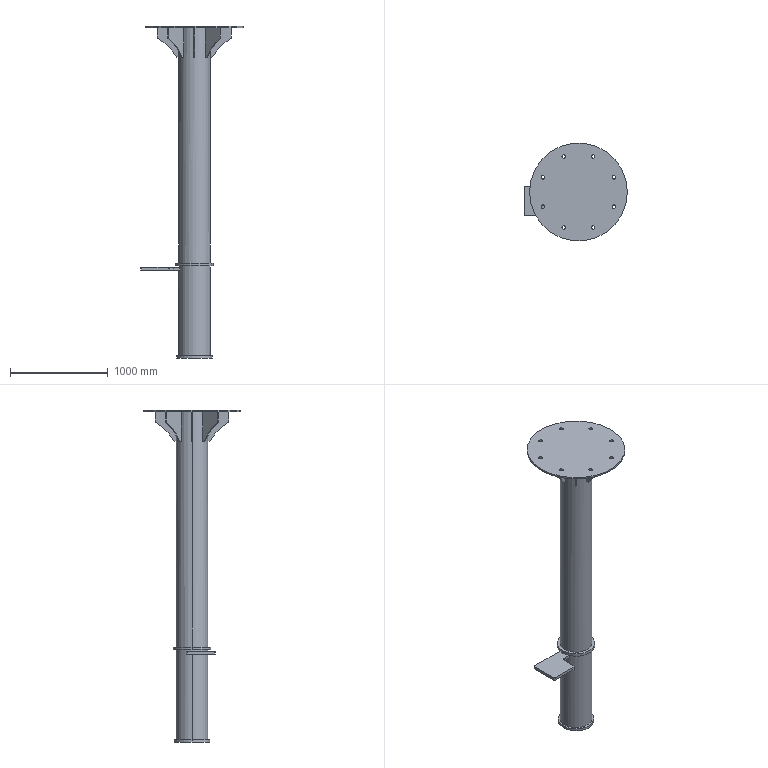Part | SolidWorks | features ICE 6, CirPattern 1, Extrusion 1 | 1 solid | 87 faces | box 1050 x 1000 x 3392 mm | volume 86673581 mm3 | plane 47 | cylinder 40 | commonest cylinder face diameters 36 x16 1134 x8 325 x4 20 x3 285 x2 365 x2